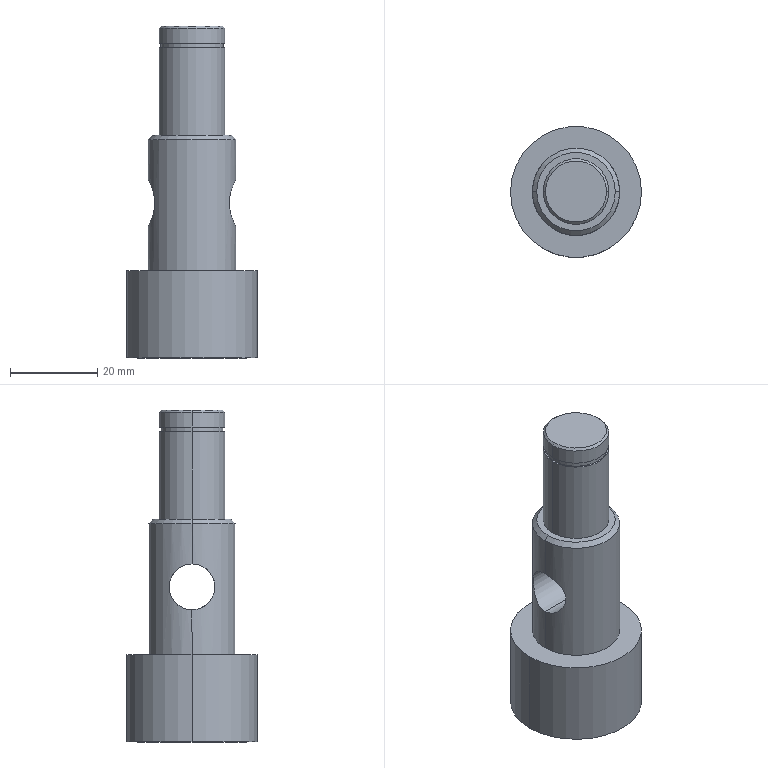Part | STEP file | Shaft end fixing piece | 1 solid | 32 faces | box 30 x 30 x 76 mm | volume 20757 mm3 | cylinder 16 | cone 8 | plane 8 | commonest cylinder face diameters 15 x4 10.5 x2 14.3 x2 18 x2 20 x2 24 x2